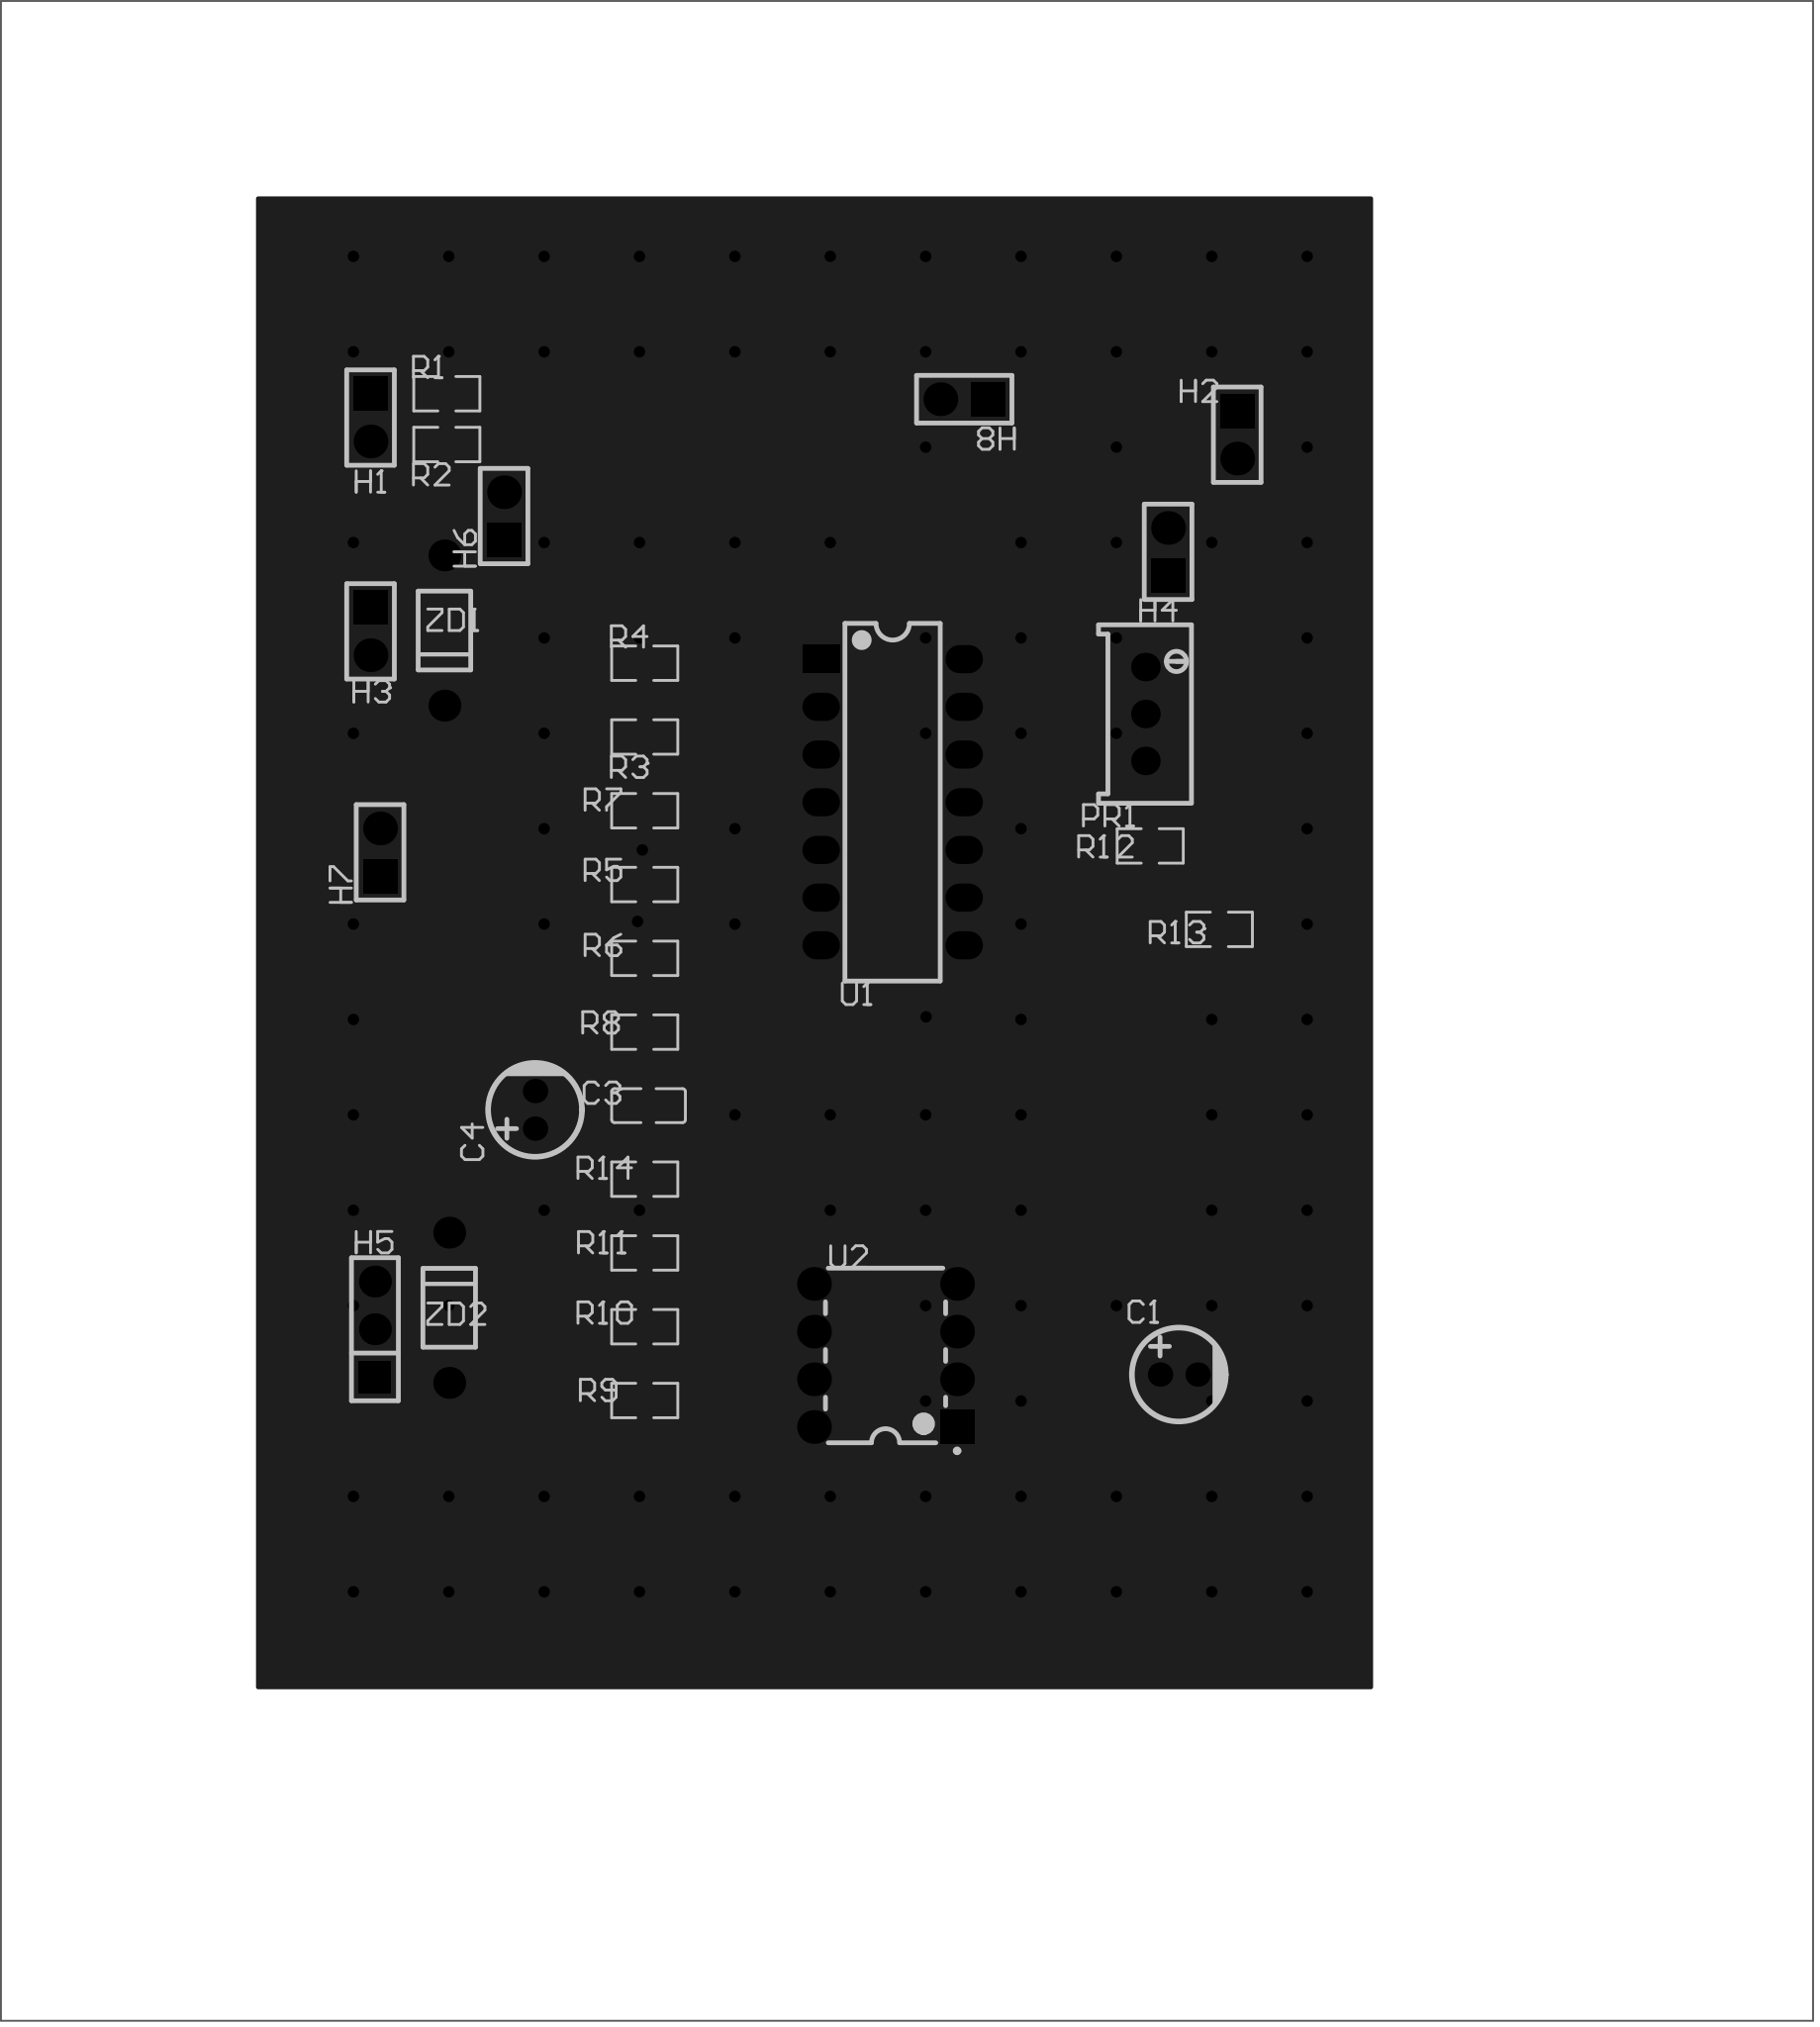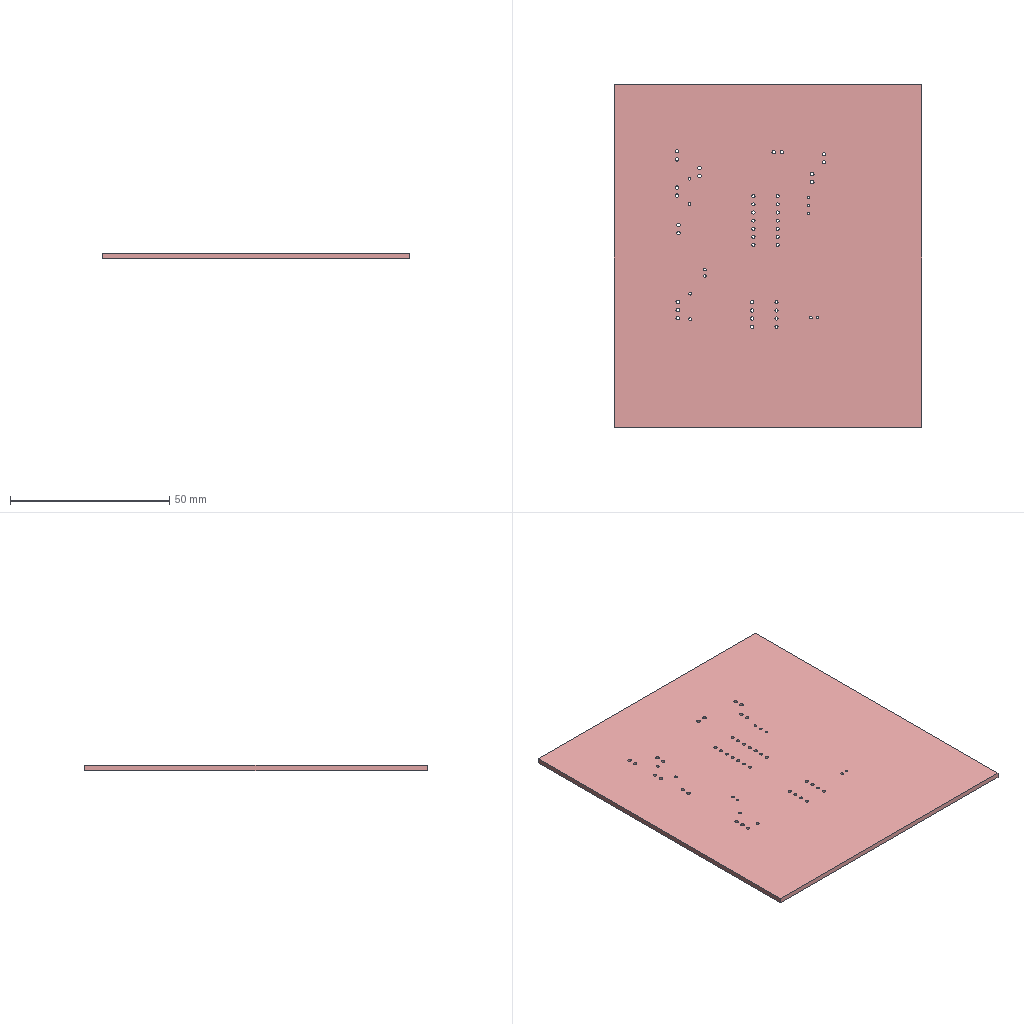Circuit board layout | Altium Designer | box 96.5 x 107.6 x 1.6 mm
Layer stack:
# Altium Designer layer stack of  (unit mm; dielectric type: 0 none, 1 core, 2 prepreg, 3 surface material)
index,name,kind,layer,copper_thickness_mm,dielectric_type,dielectric_thickness_mm,dielectric_material,dielectric_constant
0,Top Paste Mask Layer,other,,,,,,
1,Top Silkscreen Layer,other,,,,,,
2,Top Solder Mask Layer,dielectric,,,3,0.01,,3.3
3,Top Layer,copper,Top Layer,0.035,,,,
4,Dielectric1,dielectric,,,3,1.51,FR4,4.5
5,Bottom Layer,copper,Bottom Layer,0.035,,,,
6,Bottom Solder Mask Layer,dielectric,,,3,0.01,,3.3
7,Bottom Silkscreen Layer,other,,,,,,
8,Bottom Paste Mask Layer,other,,,,,,
# drill layer pairs: low layer,high layer
drill_pair,Top Layer,Bottom Layer
Part placement:
Designator,Comment,Layer,Footprint,Center-X(mm),Center-Y(mm),Rotation
C3,0.01uF,TopLayer,C0805,104.343,118.588,0
H1,,TopLayer,HDR-TH_2P-P2.54-V-M-1,89.535,155.232,270
H2,,TopLayer,HDR-TH_2P-P2.54-V-M-1,135.7,154.319,270
H3,,TopLayer,HDR-TH_2P-P2.54-V-M-1,89.535,143.847,270
H4,,TopLayer,HDR-TH_2P-P2.54-V-M-1,132.017,148.083,90
H5,,TopLayer,HDR-TH_3P-P2.54-V-M,89.769,106.68,90
PR1,5kΩ,TopLayer,R_3296,130.81,139.446,270
R1,1K,TopLayer,R0805,93.599,156.502,0
R2,100K,TopLayer,R0805,93.599,153.797,0
R3,1K,TopLayer,R0805,104.14,138.222,0
R4,10K,TopLayer,R0805,104.14,142.151,0
R5,1K,TopLayer,R0805,104.14,130.363,180
R6,100K,TopLayer,R0805,104.14,126.433,180
R7,1K,TopLayer,R0805,104.14,134.292,0
R8,1K,TopLayer,R0805,104.14,122.504,0
R9,68K,TopLayer,R0805,104.14,102.883,0
R10,10K,TopLayer,R0805,104.14,106.813,180
R11,100K,TopLayer,R0805,104.14,110.743,180
R12,12K,TopLayer,R0805,131.064,132.42,180
R13,100K,TopLayer,R0805,134.747,127.975,180
R14,6.81K,TopLayer,R0805,104.14,114.672,180
U1,LM324,TopLayer,PDIP-14_L19.3-W6.5-P2.54-LS7.6-BL,117.348,134.747,270
U2,100kHz,TopLayer,DIP-8_L9.2-W6.4-P2.54-LS7.6-BL,116.967,105.283,90
ZD1,1N4733A,TopLayer,DO-41_BD2.8-L4.2-P8.00-D0.7-FD,93.472,143.891,270
ZD2,1N4733A,TopLayer,DO-41_BD2.8-L4.2-P8.00-D0.7-FD,93.726,107.823,90
C1,1uF,TopLayer,CAP-TH_BD5.0-P2.00-D0.8-FD-10UF50VC110GL,132.588,104.267,0
C4,470pF,TopLayer,CAP-TH_BD5.0-P2.00-D0.8-FD-10UF50VC110GL,98.298,118.364,90
H7,,TopLayer,HDR-TH_2P-P2.54-V-M-1,90.043,132.08,90
H6,,TopLayer,HDR-TH_2P-P2.54-V-M-1,96.647,149.987,90
H8,,TopLayer,HDR-TH_2P-P2.54-V-M-1,121.158,156.21,180
Pad and via stacks:
# Altium Designer via and pad stacks of  (unit mm). Each distinct definition once, with the count of objects using it.
# via: kind,start_layer,end_layer,hole_mm,diameter_mm,mode(0 simple;1 top-mid-bottom;2 full stack),diameter_per_layer,count,example_net
# pad: kind,layer,hole_mm,hole_type(0 round;1 square;2 slot),plating,top_size,top_shape(1 round;2 rect;3 octagon;9 rounded rect),mid_size,bottom_size,mode,footprint,size_per_layer,count,example
pad,Top Layer,0,0,plated,1.41x1.35,2,1.41x1.35,1.41x1.35,0,C0805,,2,C3.2
pad,Top Layer,0,0,plated,1.133x1.377,2,1.133x1.377,1.133x1.377,0,R0805,,28,R1.2
pad,Multi-Layer,1.1,0,plated,1.8x1.8,1,1.8x1.8,1.8x1.8,0,HDR-TH_2P-P2.54-V-M-1,,7,H1.2
pad,Multi-Layer,1.1,0,plated,1.8x1.8,2,1.8x1.8,1.8x1.8,0,HDR-TH_2P-P2.54-V-M-1,,7,H1.1
pad,Multi-Layer,1.1,0,plated,1.7x1.7,2,1.7x1.7,1.7x1.7,0,HDR-TH_3P-P2.54-V-M,,1,H5.1
pad,Multi-Layer,1.1,0,plated,1.7x1.7,1,1.7x1.7,1.7x1.7,0,HDR-TH_3P-P2.54-V-M,,2,H5.2
pad,Multi-Layer,0.762,0,plated,1.524x1.524,1,1.524x1.524,1.524x1.524,0,R_3296,,3,PR1.2
pad,Multi-Layer,1,0,plated,1.5x2,1,1.5x2,1.5x2,0,PDIP-14_L19.3-W6.5-P2.54-LS7.6-BL,,13,U1.8
pad,Multi-Layer,1,0,plated,1.5x2,2,1.5x2,1.5x2,0,PDIP-14_L19.3-W6.5-P2.54-LS7.6-BL,,1,U1.1
pad,Multi-Layer,1,0,plated,1.8x1.8,1,1.8x1.8,1.8x1.8,0,DIP-8_L9.2-W6.4-P2.54-LS7.6-BL,,7,U2.8
pad,Multi-Layer,1,0,plated,1.8x1.8,2,1.8x1.8,1.8x1.8,0,DIP-8_L9.2-W6.4-P2.54-LS7.6-BL,,1,U2.1
pad,Multi-Layer,0.9,0,plated,1.7x1.7,1,1.7x1.7,1.7x1.7,0,DO-41_BD2.8-L4.2-P8.00-D0.7-FD,,4,ZD1.1
pad,Multi-Layer,0.8,0,plated,1.3x1.3,1,1.3x1.3,1.3x1.3,0,CAP-TH_BD5.0-P2.00-D0.8-FD-10UF50VC110GL,,4,C1.2
via,Top Layer,Bottom Layer,0.3048,0.61,0,,111,$1N13
Copper pours:
name,layer,net,type(0 solid;1 hatched;2 none)
Top Layer-GND,Top Layer,GND,0
Bottom Layer-GND,Bottom Layer,GND,0